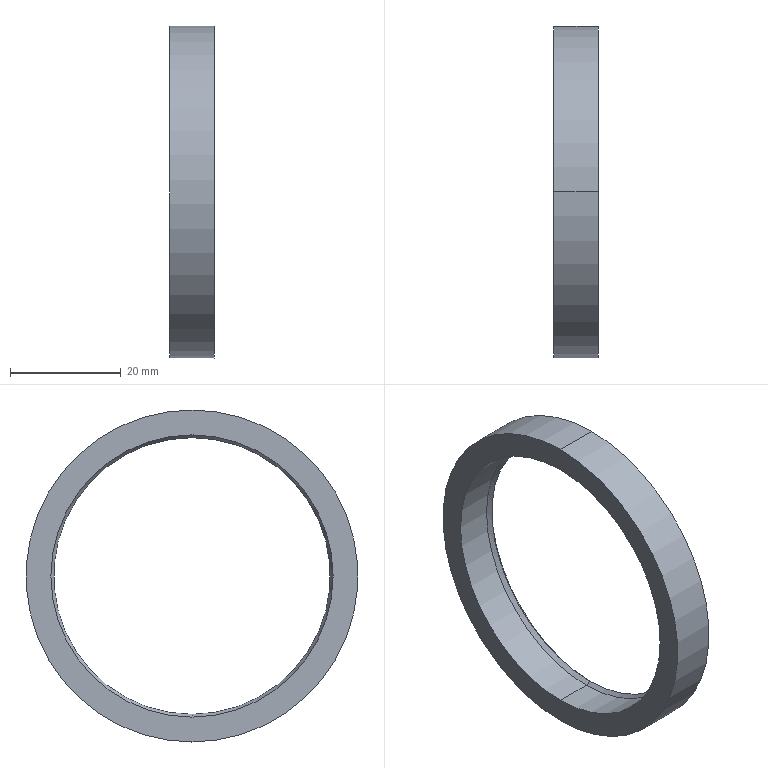Part | SolidWorks | features Revolution 2 | 1 solid | 17 faces | box 8 x 60 x 60 mm | volume 5343 mm3 | cone 8 | cylinder 4 | plane 3 | torus 2 | commonest cylinder face diameters 51 x2 60 x2
STEP:
#1=CARTESIAN_POINT('',(7.5,0.,-25.));
#2=VERTEX_POINT('',#1);
#3=CARTESIAN_POINT('',(7.5,0.,25.));
#4=VERTEX_POINT('',#3);
#5=CARTESIAN_POINT('',(7.5,0.,0.));
#6=DIRECTION('',(-1.,0.,0.));
#7=DIRECTION('',(0.,0.,1.));
#8=AXIS2_PLACEMENT_3D('',#5,#6,#7);
#9=CIRCLE('',#8,25.);
#10=EDGE_CURVE('',#2,#4,#9,.T.);
#11=ORIENTED_EDGE('',*,*,#10,.T.);
#12=CARTESIAN_POINT('',(8.,0.,25.5));
#13=VERTEX_POINT('',#12);
#14=CARTESIAN_POINT('',(7.5,0.,25.));
#15=DIRECTION('',(0.7071,0.,0.7071));
#16=VECTOR('',#15,1000.);
#17=LINE('',#14,#16);
#18=EDGE_CURVE('',#4,#13,#17,.T.);
#19=ORIENTED_EDGE('',*,*,#18,.T.);
#20=CARTESIAN_POINT('',(8.,0.,-25.5));
#21=VERTEX_POINT('',#20);
#22=CARTESIAN_POINT('',(8.,0.,0.));
#23=DIRECTION('',(-1.,0.,0.));
#24=DIRECTION('',(0.,0.,1.));
#25=AXIS2_PLACEMENT_3D('',#22,#23,#24);
#26=CIRCLE('',#25,25.5);
#27=EDGE_CURVE('',#21,#13,#26,.T.);
#28=ORIENTED_EDGE('',*,*,#27,.F.);
#29=CARTESIAN_POINT('',(7.5,0.,-25.));
#30=DIRECTION('',(0.7071,0.,-0.7071));
#31=VECTOR('',#30,1000.);
#32=LINE('',#29,#31);
#33=EDGE_CURVE('',#2,#21,#32,.T.);
#34=ORIENTED_EDGE('',*,*,#33,.F.);
#35=EDGE_LOOP('',(#11,#19,#28,#34));
#36=FACE_OUTER_BOUND('',#35,.T.);
#37=CARTESIAN_POINT('',(7.5,0.,0.));
#38=DIRECTION('',(1.,0.,0.));
#39=DIRECTION('',(0.,0.,-1.));
#40=AXIS2_PLACEMENT_3D('',#37,#38,#39);
#41=CONICAL_SURFACE('',#40,25.,0.7854);
#42=ADVANCED_FACE('',(#36),#41,.F.);
#43=ORIENTED_EDGE('',*,*,#10,.F.);
#44=CARTESIAN_POINT('',(6.634,0.,-25.5));
#45=VERTEX_POINT('',#44);
#46=CARTESIAN_POINT('',(6.634,0.,-25.5));
#47=DIRECTION('',(-0.866,0.,-0.5));
#48=VECTOR('',#47,1000.);
#49=LINE('',#46,#48);
#50=EDGE_CURVE('',#2,#45,#49,.T.);
#51=ORIENTED_EDGE('',*,*,#50,.T.);
#52=CARTESIAN_POINT('',(6.634,0.,25.5));
#53=VERTEX_POINT('',#52);
#54=CARTESIAN_POINT('',(6.634,0.,0.));
#55=DIRECTION('',(-1.,0.,0.));
#56=DIRECTION('',(0.,0.,1.));
#57=AXIS2_PLACEMENT_3D('',#54,#55,#56);
#58=CIRCLE('',#57,25.5);
#59=EDGE_CURVE('',#45,#53,#58,.T.);
#60=ORIENTED_EDGE('',*,*,#59,.T.);
#61=CARTESIAN_POINT('',(6.634,0.,25.5));
#62=DIRECTION('',(-0.866,0.,0.5));
#63=VECTOR('',#62,1000.);
#64=LINE('',#61,#63);
#65=EDGE_CURVE('',#4,#53,#64,.T.);
#66=ORIENTED_EDGE('',*,*,#65,.F.);
#67=EDGE_LOOP('',(#43,#51,#60,#66));
#68=FACE_OUTER_BOUND('',#67,.T.);
#69=CARTESIAN_POINT('',(6.634,0.,0.));
#70=DIRECTION('',(-1.,0.,0.));
#71=DIRECTION('',(0.,0.,1.));
#72=AXIS2_PLACEMENT_3D('',#69,#70,#71);
#73=CONICAL_SURFACE('',#72,25.5,0.5236);
#74=ADVANCED_FACE('',(#68),#73,.F.);
#75=ORIENTED_EDGE('',*,*,#59,.F.);
#76=CARTESIAN_POINT('',(0.,0.,-25.5));
#77=VERTEX_POINT('',#76);
#78=CARTESIAN_POINT('',(0.,0.,-25.5));
#79=DIRECTION('',(-1.,0.,0.));
#80=VECTOR('',#79,1000.);
#81=LINE('',#78,#80);
#82=EDGE_CURVE('',#45,#77,#81,.T.);
#83=ORIENTED_EDGE('',*,*,#82,.T.);
#84=CARTESIAN_POINT('',(0.,0.,25.5));
#85=VERTEX_POINT('',#84);
#86=CARTESIAN_POINT('',(0.,0.,0.));
#87=DIRECTION('',(-1.,0.,0.));
#88=DIRECTION('',(0.,0.,1.));
#89=AXIS2_PLACEMENT_3D('',#86,#87,#88);
#90=CIRCLE('',#89,25.5);
#91=EDGE_CURVE('',#77,#85,#90,.T.);
#92=ORIENTED_EDGE('',*,*,#91,.T.);
#93=CARTESIAN_POINT('',(0.,0.,25.5));
#94=DIRECTION('',(-1.,0.,0.));
#95=VECTOR('',#94,1000.);
#96=LINE('',#93,#95);
#97=EDGE_CURVE('',#53,#85,#96,.T.);
#98=ORIENTED_EDGE('',*,*,#97,.F.);
#99=EDGE_LOOP('',(#75,#83,#92,#98));
#100=FACE_OUTER_BOUND('',#99,.T.);
#101=CARTESIAN_POINT('',(0.,0.,0.));
#102=DIRECTION('',(-1.,0.,0.));
#103=DIRECTION('',(0.,0.,1.));
#104=AXIS2_PLACEMENT_3D('',#101,#102,#103);
#105=CYLINDRICAL_SURFACE('',#104,25.5);
#106=ADVANCED_FACE('',(#100),#105,.F.);
#107=CARTESIAN_POINT('',(8.,0.,30.));
#108=VERTEX_POINT('',#107);
#109=CARTESIAN_POINT('',(8.,0.,-30.));
#110=VERTEX_POINT('',#109);
#111=CARTESIAN_POINT('',(8.,0.,0.));
#112=DIRECTION('',(-1.,0.,0.));
#113=DIRECTION('',(0.,0.,1.));
#114=AXIS2_PLACEMENT_3D('',#111,#112,#113);
#115=CIRCLE('',#114,30.);
#116=EDGE_CURVE('',#108,#110,#115,.T.);
#117=ORIENTED_EDGE('',*,*,#116,.T.);
#118=CARTESIAN_POINT('',(0.,0.,-30.));
#119=VERTEX_POINT('',#118);
#120=CARTESIAN_POINT('',(0.,0.,-30.));
#121=DIRECTION('',(-1.,0.,0.));
#122=VECTOR('',#121,1000.);
#123=LINE('',#120,#122);
#124=EDGE_CURVE('',#110,#119,#123,.T.);
#125=ORIENTED_EDGE('',*,*,#124,.T.);
#126=CARTESIAN_POINT('',(0.,0.,30.));
#127=VERTEX_POINT('',#126);
#128=CARTESIAN_POINT('',(0.,0.,0.));
#129=DIRECTION('',(-1.,0.,0.));
#130=DIRECTION('',(0.,0.,1.));
#131=AXIS2_PLACEMENT_3D('',#128,#129,#130);
#132=CIRCLE('',#131,30.);
#133=EDGE_CURVE('',#127,#119,#132,.T.);
#134=ORIENTED_EDGE('',*,*,#133,.F.);
#135=CARTESIAN_POINT('',(0.,0.,30.));
#136=DIRECTION('',(-1.,0.,0.));
#137=VECTOR('',#136,1000.);
#138=LINE('',#135,#137);
#139=EDGE_CURVE('',#108,#127,#138,.T.);
#140=ORIENTED_EDGE('',*,*,#139,.F.);
#141=EDGE_LOOP('',(#117,#125,#134,#140));
#142=FACE_OUTER_BOUND('',#141,.T.);
#143=CARTESIAN_POINT('',(0.,0.,0.));
#144=DIRECTION('',(-1.,0.,0.));
#145=DIRECTION('',(0.,0.,1.));
#146=AXIS2_PLACEMENT_3D('',#143,#144,#145);
#147=CYLINDRICAL_SURFACE('',#146,30.);
#148=ADVANCED_FACE('',(#142),#147,.T.);
#149=CARTESIAN_POINT('',(3.926,0.,-27.825));
#150=VERTEX_POINT('',#149);
#151=CARTESIAN_POINT('',(3.926,0.,27.825));
#152=VERTEX_POINT('',#151);
#153=CARTESIAN_POINT('',(3.926,0.,0.));
#154=DIRECTION('',(-1.,0.,0.));
#155=DIRECTION('',(0.,0.,1.));
#156=AXIS2_PLACEMENT_3D('',#153,#154,#155);
#157=CIRCLE('',#156,27.825);
#158=EDGE_CURVE('',#150,#152,#157,.T.);
#159=ORIENTED_EDGE('',*,*,#158,.T.);
#160=CARTESIAN_POINT('',(8.,0.,28.75));
#161=VERTEX_POINT('',#160);
#162=CARTESIAN_POINT('',(8.,0.,28.75));
#163=DIRECTION('',(0.9752,0.,0.2214));
#164=VECTOR('',#163,1000.);
#165=LINE('',#162,#164);
#166=EDGE_CURVE('',#152,#161,#165,.T.);
#167=ORIENTED_EDGE('',*,*,#166,.T.);
#168=CARTESIAN_POINT('',(8.,0.,-28.75));
#169=VERTEX_POINT('',#168);
#170=CARTESIAN_POINT('',(8.,0.,0.));
#171=DIRECTION('',(-1.,0.,0.));
#172=DIRECTION('',(0.,0.,1.));
#173=AXIS2_PLACEMENT_3D('',#170,#171,#172);
#174=CIRCLE('',#173,28.75);
#175=EDGE_CURVE('',#169,#161,#174,.T.);
#176=ORIENTED_EDGE('',*,*,#175,.F.);
#177=CARTESIAN_POINT('',(8.,0.,-28.75));
#178=DIRECTION('',(0.9752,0.,-0.2214));
#179=VECTOR('',#178,1000.);
#180=LINE('',#177,#179);
#181=EDGE_CURVE('',#150,#169,#180,.T.);
#182=ORIENTED_EDGE('',*,*,#181,.F.);
#183=EDGE_LOOP('',(#159,#167,#176,#182));
#184=FACE_OUTER_BOUND('',#183,.T.);
#185=CARTESIAN_POINT('',(8.,0.,0.));
#186=DIRECTION('',(1.,0.,0.));
#187=DIRECTION('',(0.,0.,-1.));
#188=AXIS2_PLACEMENT_3D('',#185,#186,#187);
#189=CONICAL_SURFACE('',#188,28.75,0.2233);
#190=ADVANCED_FACE('',(#184),#189,.F.);
#191=ORIENTED_EDGE('',*,*,#158,.F.);
#192=CARTESIAN_POINT('',(3.959,0.,-27.169));
#193=VERTEX_POINT('',#192);
#194=CARTESIAN_POINT('',(4.,0.,-27.5));
#195=DIRECTION('',(0.,1.,0.));
#196=DIRECTION('',(-1.,0.,0.));
#197=AXIS2_PLACEMENT_3D('',#194,#195,#196);
#198=CIRCLE('',#197,0.3333);
#199=EDGE_CURVE('',#150,#193,#198,.T.);
#200=ORIENTED_EDGE('',*,*,#199,.T.);
#201=CARTESIAN_POINT('',(3.959,0.,27.169));
#202=VERTEX_POINT('',#201);
#203=CARTESIAN_POINT('',(3.959,0.,0.));
#204=DIRECTION('',(-1.,0.,0.));
#205=DIRECTION('',(0.,0.,1.));
#206=AXIS2_PLACEMENT_3D('',#203,#204,#205);
#207=CIRCLE('',#206,27.169);
#208=EDGE_CURVE('',#193,#202,#207,.T.);
#209=ORIENTED_EDGE('',*,*,#208,.T.);
#210=CARTESIAN_POINT('',(4.,0.,27.5));
#211=DIRECTION('',(0.,-1.,0.));
#212=DIRECTION('',(1.,0.,0.));
#213=AXIS2_PLACEMENT_3D('',#210,#211,#212);
#214=CIRCLE('',#213,0.3333);
#215=EDGE_CURVE('',#152,#202,#214,.T.);
#216=ORIENTED_EDGE('',*,*,#215,.F.);
#217=EDGE_LOOP('',(#191,#200,#209,#216));
#218=FACE_OUTER_BOUND('',#217,.T.);
#219=CARTESIAN_POINT('',(4.,0.,0.));
#220=DIRECTION('',(-1.,0.,0.));
#221=DIRECTION('',(0.,0.,1.));
#222=AXIS2_PLACEMENT_3D('',#219,#220,#221);
#223=TOROIDAL_SURFACE('',#222,27.5,0.3333);
#224=ADVANCED_FACE('',(#218),#223,.F.);
#225=CARTESIAN_POINT('',(8.,0.,26.667));
#226=VERTEX_POINT('',#225);
#227=CARTESIAN_POINT('',(8.,0.,-26.667));
#228=VERTEX_POINT('',#227);
#229=CARTESIAN_POINT('',(8.,0.,0.));
#230=DIRECTION('',(-1.,0.,0.));
#231=DIRECTION('',(0.,0.,1.));
#232=AXIS2_PLACEMENT_3D('',#229,#230,#231);
#233=CIRCLE('',#232,26.667);
#234=EDGE_CURVE('',#226,#228,#233,.T.);
#235=ORIENTED_EDGE('',*,*,#234,.T.);
#236=CARTESIAN_POINT('',(3.959,0.,-27.169));
#237=DIRECTION('',(-0.9924,0.,-0.1234));
#238=VECTOR('',#237,1000.);
#239=LINE('',#236,#238);
#240=EDGE_CURVE('',#228,#193,#239,.T.);
#241=ORIENTED_EDGE('',*,*,#240,.T.);
#242=CARTESIAN_POINT('',(3.959,0.,0.));
#243=DIRECTION('',(-1.,0.,0.));
#244=DIRECTION('',(0.,0.,1.));
#245=AXIS2_PLACEMENT_3D('',#242,#243,#244);
#246=CIRCLE('',#245,27.169);
#247=EDGE_CURVE('',#202,#193,#246,.T.);
#248=ORIENTED_EDGE('',*,*,#247,.F.);
#249=CARTESIAN_POINT('',(3.959,0.,27.169));
#250=DIRECTION('',(-0.9924,0.,0.1234));
#251=VECTOR('',#250,1000.);
#252=LINE('',#249,#251);
#253=EDGE_CURVE('',#226,#202,#252,.T.);
#254=ORIENTED_EDGE('',*,*,#253,.F.);
#255=EDGE_LOOP('',(#235,#241,#248,#254));
#256=FACE_OUTER_BOUND('',#255,.T.);
#257=CARTESIAN_POINT('',(3.959,0.,0.));
#258=DIRECTION('',(-1.,0.,0.));
#259=DIRECTION('',(0.,0.,1.));
#260=AXIS2_PLACEMENT_3D('',#257,#258,#259);
#261=CONICAL_SURFACE('',#260,27.169,0.1237);
#262=ADVANCED_FACE('',(#256),#261,.T.);
#263=ORIENTED_EDGE('',*,*,#240,.F.);
#264=CARTESIAN_POINT('',(8.,0.,0.));
#265=DIRECTION('',(-1.,0.,0.));
#266=DIRECTION('',(0.,0.,1.));
#267=AXIS2_PLACEMENT_3D('',#264,#265,#266);
#268=CIRCLE('',#267,26.667);
#269=EDGE_CURVE('',#228,#226,#268,.T.);
#270=ORIENTED_EDGE('',*,*,#269,.T.);
#271=ORIENTED_EDGE('',*,*,#253,.T.);
#272=ORIENTED_EDGE('',*,*,#208,.F.);
#273=EDGE_LOOP('',(#263,#270,#271,#272));
#274=FACE_OUTER_BOUND('',#273,.T.);
#275=CARTESIAN_POINT('',(3.959,0.,0.));
#276=DIRECTION('',(-1.,0.,0.));
#277=DIRECTION('',(0.,0.,1.));
#278=AXIS2_PLACEMENT_3D('',#275,#276,#277);
#279=CONICAL_SURFACE('',#278,27.169,0.1237);
#280=ADVANCED_FACE('',(#274),#279,.T.);
#281=ORIENTED_EDGE('',*,*,#199,.F.);
#282=CARTESIAN_POINT('',(3.926,0.,0.));
#283=DIRECTION('',(-1.,0.,0.));
#284=DIRECTION('',(0.,0.,1.));
#285=AXIS2_PLACEMENT_3D('',#282,#283,#284);
#286=CIRCLE('',#285,27.825);
#287=EDGE_CURVE('',#152,#150,#286,.T.);
#288=ORIENTED_EDGE('',*,*,#287,.F.);
#289=ORIENTED_EDGE('',*,*,#215,.T.);
#290=ORIENTED_EDGE('',*,*,#247,.T.);
#291=EDGE_LOOP('',(#281,#288,#289,#290));
#292=FACE_OUTER_BOUND('',#291,.T.);
#293=CARTESIAN_POINT('',(4.,0.,0.));
#294=DIRECTION('',(-1.,0.,0.));
#295=DIRECTION('',(0.,0.,1.));
#296=AXIS2_PLACEMENT_3D('',#293,#294,#295);
#297=TOROIDAL_SURFACE('',#296,27.5,0.3333);
#298=ADVANCED_FACE('',(#292),#297,.F.);
#299=ORIENTED_EDGE('',*,*,#166,.F.);
#300=ORIENTED_EDGE('',*,*,#287,.T.);
#301=ORIENTED_EDGE('',*,*,#181,.T.);
#302=CARTESIAN_POINT('',(8.,0.,0.));
#303=DIRECTION('',(-1.,0.,0.));
#304=DIRECTION('',(0.,0.,1.));
#305=AXIS2_PLACEMENT_3D('',#302,#303,#304);
#306=CIRCLE('',#305,28.75);
#307=EDGE_CURVE('',#161,#169,#306,.T.);
#308=ORIENTED_EDGE('',*,*,#307,.F.);
#309=EDGE_LOOP('',(#299,#300,#301,#308));
#310=FACE_OUTER_BOUND('',#309,.T.);
#311=CARTESIAN_POINT('',(8.,0.,0.));
#312=DIRECTION('',(1.,0.,0.));
#313=DIRECTION('',(0.,0.,-1.));
#314=AXIS2_PLACEMENT_3D('',#311,#312,#313);
#315=CONICAL_SURFACE('',#314,28.75,0.2233);
#316=ADVANCED_FACE('',(#310),#315,.F.);
#317=ORIENTED_EDGE('',*,*,#175,.T.);
#318=ORIENTED_EDGE('',*,*,#307,.T.);
#319=EDGE_LOOP('',(#317,#318));
#320=FACE_BOUND('',#319,.T.);
#321=ORIENTED_EDGE('',*,*,#116,.F.);
#322=CARTESIAN_POINT('',(8.,0.,0.));
#323=DIRECTION('',(-1.,0.,0.));
#324=DIRECTION('',(0.,0.,1.));
#325=AXIS2_PLACEMENT_3D('',#322,#323,#324);
#326=CIRCLE('',#325,30.);
#327=EDGE_CURVE('',#110,#108,#326,.T.);
#328=ORIENTED_EDGE('',*,*,#327,.F.);
#329=EDGE_LOOP('',(#321,#328));
#330=FACE_OUTER_BOUND('',#329,.T.);
#331=CARTESIAN_POINT('',(8.,0.,0.));
#332=DIRECTION('',(1.,0.,0.));
#333=DIRECTION('',(0.,0.,-1.));
#334=AXIS2_PLACEMENT_3D('',#331,#332,#333);
#335=PLANE('',#334);
#336=ADVANCED_FACE('',(#320,#330),#335,.T.);
#337=ORIENTED_EDGE('',*,*,#124,.F.);
#338=ORIENTED_EDGE('',*,*,#327,.T.);
#339=ORIENTED_EDGE('',*,*,#139,.T.);
#340=CARTESIAN_POINT('',(0.,0.,0.));
#341=DIRECTION('',(-1.,0.,0.));
#342=DIRECTION('',(0.,0.,1.));
#343=AXIS2_PLACEMENT_3D('',#340,#341,#342);
#344=CIRCLE('',#343,30.);
#345=EDGE_CURVE('',#119,#127,#344,.T.);
#346=ORIENTED_EDGE('',*,*,#345,.F.);
#347=EDGE_LOOP('',(#337,#338,#339,#346));
#348=FACE_OUTER_BOUND('',#347,.T.);
#349=CARTESIAN_POINT('',(0.,0.,0.));
#350=DIRECTION('',(-1.,0.,0.));
#351=DIRECTION('',(0.,0.,1.));
#352=AXIS2_PLACEMENT_3D('',#349,#350,#351);
#353=CYLINDRICAL_SURFACE('',#352,30.);
#354=ADVANCED_FACE('',(#348),#353,.T.);
#355=ORIENTED_EDGE('',*,*,#133,.T.);
#356=ORIENTED_EDGE('',*,*,#345,.T.);
#357=EDGE_LOOP('',(#355,#356));
#358=FACE_OUTER_BOUND('',#357,.T.);
#359=CARTESIAN_POINT('',(0.,0.,0.));
#360=DIRECTION('',(-1.,0.,0.));
#361=DIRECTION('',(0.,0.,1.));
#362=AXIS2_PLACEMENT_3D('',#359,#360,#361);
#363=CIRCLE('',#362,25.5);
#364=EDGE_CURVE('',#85,#77,#363,.T.);
#365=ORIENTED_EDGE('',*,*,#364,.F.);
#366=ORIENTED_EDGE('',*,*,#91,.F.);
#367=EDGE_LOOP('',(#365,#366));
#368=FACE_BOUND('',#367,.T.);
#369=CARTESIAN_POINT('',(0.,0.,0.));
#370=DIRECTION('',(-1.,0.,0.));
#371=DIRECTION('',(0.,0.,1.));
#372=AXIS2_PLACEMENT_3D('',#369,#370,#371);
#373=PLANE('',#372);
#374=ADVANCED_FACE('',(#358,#368),#373,.T.);
#375=ORIENTED_EDGE('',*,*,#82,.F.);
#376=CARTESIAN_POINT('',(6.634,0.,0.));
#377=DIRECTION('',(-1.,0.,0.));
#378=DIRECTION('',(0.,0.,1.));
#379=AXIS2_PLACEMENT_3D('',#376,#377,#378);
#380=CIRCLE('',#379,25.5);
#381=EDGE_CURVE('',#53,#45,#380,.T.);
#382=ORIENTED_EDGE('',*,*,#381,.F.);
#383=ORIENTED_EDGE('',*,*,#97,.T.);
#384=ORIENTED_EDGE('',*,*,#364,.T.);
#385=EDGE_LOOP('',(#375,#382,#383,#384));
#386=FACE_OUTER_BOUND('',#385,.T.);
#387=CARTESIAN_POINT('',(0.,0.,0.));
#388=DIRECTION('',(-1.,0.,0.));
#389=DIRECTION('',(0.,0.,1.));
#390=AXIS2_PLACEMENT_3D('',#387,#388,#389);
#391=CYLINDRICAL_SURFACE('',#390,25.5);
#392=ADVANCED_FACE('',(#386),#391,.F.);
#393=ORIENTED_EDGE('',*,*,#50,.F.);
#394=CARTESIAN_POINT('',(7.5,0.,0.));
#395=DIRECTION('',(-1.,0.,0.));
#396=DIRECTION('',(0.,0.,1.));
#397=AXIS2_PLACEMENT_3D('',#394,#395,#396);
#398=CIRCLE('',#397,25.);
#399=EDGE_CURVE('',#4,#2,#398,.T.);
#400=ORIENTED_EDGE('',*,*,#399,.F.);
#401=ORIENTED_EDGE('',*,*,#65,.T.);
#402=ORIENTED_EDGE('',*,*,#381,.T.);
#403=EDGE_LOOP('',(#393,#400,#401,#402));
#404=FACE_OUTER_BOUND('',#403,.T.);
#405=CARTESIAN_POINT('',(6.634,0.,0.));
#406=DIRECTION('',(-1.,0.,0.));
#407=DIRECTION('',(0.,0.,1.));
#408=AXIS2_PLACEMENT_3D('',#405,#406,#407);
#409=CONICAL_SURFACE('',#408,25.5,0.5236);
#410=ADVANCED_FACE('',(#404),#409,.F.);
#411=ORIENTED_EDGE('',*,*,#18,.F.);
#412=ORIENTED_EDGE('',*,*,#399,.T.);
#413=ORIENTED_EDGE('',*,*,#33,.T.);
#414=CARTESIAN_POINT('',(8.,0.,0.));
#415=DIRECTION('',(-1.,0.,0.));
#416=DIRECTION('',(0.,0.,1.));
#417=AXIS2_PLACEMENT_3D('',#414,#415,#416);
#418=CIRCLE('',#417,25.5);
#419=EDGE_CURVE('',#13,#21,#418,.T.);
#420=ORIENTED_EDGE('',*,*,#419,.F.);
#421=EDGE_LOOP('',(#411,#412,#413,#420));
#422=FACE_OUTER_BOUND('',#421,.T.);
#423=CARTESIAN_POINT('',(7.5,0.,0.));
#424=DIRECTION('',(1.,0.,0.));
#425=DIRECTION('',(0.,0.,-1.));
#426=AXIS2_PLACEMENT_3D('',#423,#424,#425);
#427=CONICAL_SURFACE('',#426,25.,0.7854);
#428=ADVANCED_FACE('',(#422),#427,.F.);
#429=ORIENTED_EDGE('',*,*,#27,.T.);
#430=ORIENTED_EDGE('',*,*,#419,.T.);
#431=EDGE_LOOP('',(#429,#430));
#432=FACE_BOUND('',#431,.T.);
#433=ORIENTED_EDGE('',*,*,#234,.F.);
#434=ORIENTED_EDGE('',*,*,#269,.F.);
#435=EDGE_LOOP('',(#433,#434));
#436=FACE_OUTER_BOUND('',#435,.T.);
#437=CARTESIAN_POINT('',(8.,0.,0.));
#438=DIRECTION('',(1.,0.,0.));
#439=DIRECTION('',(0.,0.,-1.));
#440=AXIS2_PLACEMENT_3D('',#437,#438,#439);
#441=PLANE('',#440);
#442=ADVANCED_FACE('',(#432,#436),#441,.T.);
#443=CLOSED_SHELL('',(#42,#74,#106,#148,#190,#224,#262,#280,#298,#316,#336,#354,#374,#392,#410,#428,#442));
#444=MANIFOLD_SOLID_BREP('',#443);
#445=CARTESIAN_POINT('',(0.,0.,0.));
#446=DIRECTION('',(0.,0.,1.));
#447=DIRECTION('',(1.,0.,0.));
#448=AXIS2_PLACEMENT_3D('',#445,#446,#447);
#449=(LENGTH_UNIT()NAMED_UNIT(*)SI_UNIT(.MILLI.,.METRE.));
#450=UNCERTAINTY_MEASURE_WITH_UNIT(LENGTH_MEASURE(0.00001),#449,'','');
#451=(NAMED_UNIT(*)PLANE_ANGLE_UNIT()SI_UNIT($,.RADIAN.));
#452=(NAMED_UNIT(*)SI_UNIT($,.STERADIAN.)SOLID_ANGLE_UNIT());
#453=(GEOMETRIC_REPRESENTATION_CONTEXT(3)GLOBAL_UNCERTAINTY_ASSIGNED_CONTEXT((#450))GLOBAL_UNIT_ASSIGNED_CONTEXT((#449,#451,#452))REPRESENTATION_CONTEXT('',''));
#454=ADVANCED_BREP_SHAPE_REPRESENTATION('',(#444,#448),#453);